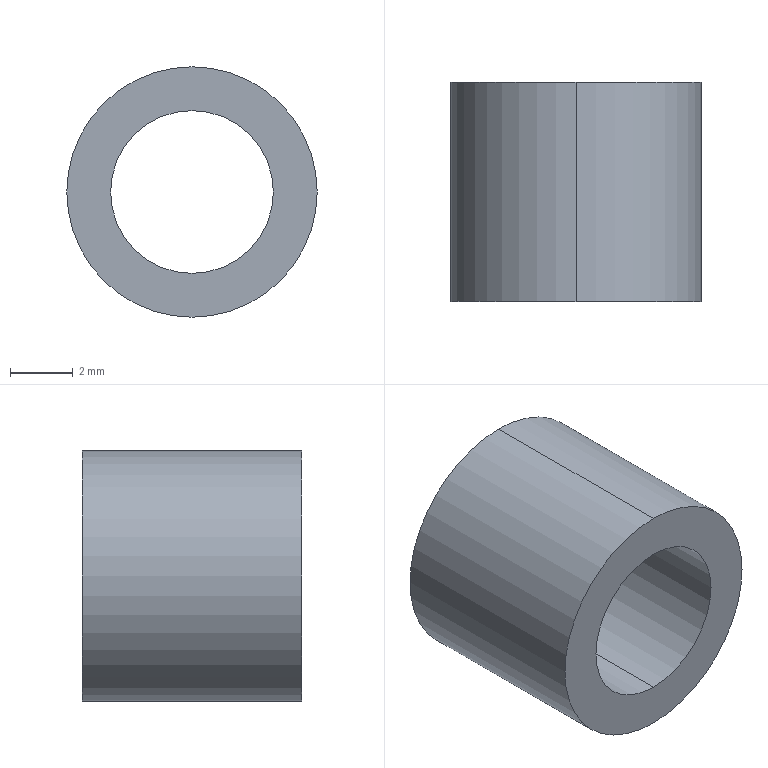Part | SolidWorks | features Extrusion 1 | 1 solid | 6 faces | box 8 x 7 x 8 mm | volume 203.198 mm3 | cylinder 4 | plane 2 | commonest cylinder face diameters 5.2 x2 8 x2
STEP:
#1=CARTESIAN_POINT('',(0.,7.,-2.6));
#2=VERTEX_POINT('',#1);
#3=CARTESIAN_POINT('',(0.,7.,2.6));
#4=VERTEX_POINT('',#3);
#5=CARTESIAN_POINT('',(0.,7.,0.));
#6=DIRECTION('',(0.,1.,0.));
#7=DIRECTION('',(0.,0.,1.));
#8=AXIS2_PLACEMENT_3D('',#5,#6,#7);
#9=CIRCLE('',#8,2.6);
#10=EDGE_CURVE('',#2,#4,#9,.T.);
#11=ORIENTED_EDGE('',*,*,#10,.T.);
#12=CARTESIAN_POINT('',(0.,0.,2.6));
#13=VERTEX_POINT('',#12);
#14=CARTESIAN_POINT('',(0.,7.,2.6));
#15=DIRECTION('',(0.,-1.,0.));
#16=VECTOR('',#15,1000.);
#17=LINE('',#14,#16);
#18=EDGE_CURVE('',#4,#13,#17,.T.);
#19=ORIENTED_EDGE('',*,*,#18,.T.);
#20=CARTESIAN_POINT('',(0.,0.,-2.6));
#21=VERTEX_POINT('',#20);
#22=CARTESIAN_POINT('',(0.,0.,0.));
#23=DIRECTION('',(0.,1.,0.));
#24=DIRECTION('',(0.,0.,1.));
#25=AXIS2_PLACEMENT_3D('',#22,#23,#24);
#26=CIRCLE('',#25,2.6);
#27=EDGE_CURVE('',#21,#13,#26,.T.);
#28=ORIENTED_EDGE('',*,*,#27,.F.);
#29=CARTESIAN_POINT('',(0.,7.,-2.6));
#30=DIRECTION('',(0.,-1.,0.));
#31=VECTOR('',#30,1000.);
#32=LINE('',#29,#31);
#33=EDGE_CURVE('',#2,#21,#32,.T.);
#34=ORIENTED_EDGE('',*,*,#33,.F.);
#35=EDGE_LOOP('',(#11,#19,#28,#34));
#36=FACE_OUTER_BOUND('',#35,.T.);
#37=CARTESIAN_POINT('',(0.,7.,0.));
#38=DIRECTION('',(0.,-1.,0.));
#39=DIRECTION('',(0.,0.,-1.));
#40=AXIS2_PLACEMENT_3D('',#37,#38,#39);
#41=CYLINDRICAL_SURFACE('',#40,2.6);
#42=ADVANCED_FACE('',(#36),#41,.F.);
#43=CARTESIAN_POINT('',(0.,7.,4.));
#44=VERTEX_POINT('',#43);
#45=CARTESIAN_POINT('',(0.,7.,-4.));
#46=VERTEX_POINT('',#45);
#47=CARTESIAN_POINT('',(0.,7.,0.));
#48=DIRECTION('',(0.,1.,0.));
#49=DIRECTION('',(0.,0.,1.));
#50=AXIS2_PLACEMENT_3D('',#47,#48,#49);
#51=CIRCLE('',#50,4.);
#52=EDGE_CURVE('',#44,#46,#51,.T.);
#53=ORIENTED_EDGE('',*,*,#52,.F.);
#54=CARTESIAN_POINT('',(0.,0.,4.));
#55=VERTEX_POINT('',#54);
#56=CARTESIAN_POINT('',(0.,7.,4.));
#57=DIRECTION('',(0.,-1.,0.));
#58=VECTOR('',#57,1000.);
#59=LINE('',#56,#58);
#60=EDGE_CURVE('',#44,#55,#59,.T.);
#61=ORIENTED_EDGE('',*,*,#60,.T.);
#62=CARTESIAN_POINT('',(0.,0.,-4.));
#63=VERTEX_POINT('',#62);
#64=CARTESIAN_POINT('',(0.,0.,0.));
#65=DIRECTION('',(0.,1.,0.));
#66=DIRECTION('',(0.,0.,1.));
#67=AXIS2_PLACEMENT_3D('',#64,#65,#66);
#68=CIRCLE('',#67,4.);
#69=EDGE_CURVE('',#55,#63,#68,.T.);
#70=ORIENTED_EDGE('',*,*,#69,.T.);
#71=CARTESIAN_POINT('',(0.,7.,-4.));
#72=DIRECTION('',(0.,-1.,0.));
#73=VECTOR('',#72,1000.);
#74=LINE('',#71,#73);
#75=EDGE_CURVE('',#46,#63,#74,.T.);
#76=ORIENTED_EDGE('',*,*,#75,.F.);
#77=EDGE_LOOP('',(#53,#61,#70,#76));
#78=FACE_OUTER_BOUND('',#77,.T.);
#79=CARTESIAN_POINT('',(0.,7.,0.));
#80=DIRECTION('',(0.,-1.,0.));
#81=DIRECTION('',(0.,0.,-1.));
#82=AXIS2_PLACEMENT_3D('',#79,#80,#81);
#83=CYLINDRICAL_SURFACE('',#82,4.);
#84=ADVANCED_FACE('',(#78),#83,.T.);
#85=CARTESIAN_POINT('',(0.,7.,0.));
#86=DIRECTION('',(0.,1.,0.));
#87=DIRECTION('',(0.,0.,1.));
#88=AXIS2_PLACEMENT_3D('',#85,#86,#87);
#89=CIRCLE('',#88,4.);
#90=EDGE_CURVE('',#46,#44,#89,.T.);
#91=ORIENTED_EDGE('',*,*,#90,.T.);
#92=ORIENTED_EDGE('',*,*,#52,.T.);
#93=EDGE_LOOP('',(#91,#92));
#94=FACE_OUTER_BOUND('',#93,.T.);
#95=ORIENTED_EDGE('',*,*,#10,.F.);
#96=CARTESIAN_POINT('',(0.,7.,0.));
#97=DIRECTION('',(0.,1.,0.));
#98=DIRECTION('',(0.,0.,1.));
#99=AXIS2_PLACEMENT_3D('',#96,#97,#98);
#100=CIRCLE('',#99,2.6);
#101=EDGE_CURVE('',#4,#2,#100,.T.);
#102=ORIENTED_EDGE('',*,*,#101,.F.);
#103=EDGE_LOOP('',(#95,#102));
#104=FACE_BOUND('',#103,.T.);
#105=CARTESIAN_POINT('',(0.,7.,0.));
#106=DIRECTION('',(0.,1.,0.));
#107=DIRECTION('',(0.,0.,1.));
#108=AXIS2_PLACEMENT_3D('',#105,#106,#107);
#109=PLANE('',#108);
#110=ADVANCED_FACE('',(#94,#104),#109,.T.);
#111=CARTESIAN_POINT('',(0.,0.,0.));
#112=DIRECTION('',(0.,1.,0.));
#113=DIRECTION('',(0.,0.,1.));
#114=AXIS2_PLACEMENT_3D('',#111,#112,#113);
#115=CIRCLE('',#114,4.);
#116=EDGE_CURVE('',#63,#55,#115,.T.);
#117=ORIENTED_EDGE('',*,*,#116,.F.);
#118=ORIENTED_EDGE('',*,*,#69,.F.);
#119=EDGE_LOOP('',(#117,#118));
#120=FACE_OUTER_BOUND('',#119,.T.);
#121=ORIENTED_EDGE('',*,*,#27,.T.);
#122=CARTESIAN_POINT('',(0.,0.,0.));
#123=DIRECTION('',(0.,1.,0.));
#124=DIRECTION('',(0.,0.,1.));
#125=AXIS2_PLACEMENT_3D('',#122,#123,#124);
#126=CIRCLE('',#125,2.6);
#127=EDGE_CURVE('',#13,#21,#126,.T.);
#128=ORIENTED_EDGE('',*,*,#127,.T.);
#129=EDGE_LOOP('',(#121,#128));
#130=FACE_BOUND('',#129,.T.);
#131=CARTESIAN_POINT('',(0.,0.,0.));
#132=DIRECTION('',(0.,1.,0.));
#133=DIRECTION('',(0.,0.,1.));
#134=AXIS2_PLACEMENT_3D('',#131,#132,#133);
#135=PLANE('',#134);
#136=ADVANCED_FACE('',(#120,#130),#135,.F.);
#137=ORIENTED_EDGE('',*,*,#60,.F.);
#138=ORIENTED_EDGE('',*,*,#90,.F.);
#139=ORIENTED_EDGE('',*,*,#75,.T.);
#140=ORIENTED_EDGE('',*,*,#116,.T.);
#141=EDGE_LOOP('',(#137,#138,#139,#140));
#142=FACE_OUTER_BOUND('',#141,.T.);
#143=CARTESIAN_POINT('',(0.,7.,0.));
#144=DIRECTION('',(0.,-1.,0.));
#145=DIRECTION('',(0.,0.,-1.));
#146=AXIS2_PLACEMENT_3D('',#143,#144,#145);
#147=CYLINDRICAL_SURFACE('',#146,4.);
#148=ADVANCED_FACE('',(#142),#147,.T.);
#149=ORIENTED_EDGE('',*,*,#18,.F.);
#150=ORIENTED_EDGE('',*,*,#101,.T.);
#151=ORIENTED_EDGE('',*,*,#33,.T.);
#152=ORIENTED_EDGE('',*,*,#127,.F.);
#153=EDGE_LOOP('',(#149,#150,#151,#152));
#154=FACE_OUTER_BOUND('',#153,.T.);
#155=CARTESIAN_POINT('',(0.,7.,0.));
#156=DIRECTION('',(0.,-1.,0.));
#157=DIRECTION('',(0.,0.,-1.));
#158=AXIS2_PLACEMENT_3D('',#155,#156,#157);
#159=CYLINDRICAL_SURFACE('',#158,2.6);
#160=ADVANCED_FACE('',(#154),#159,.F.);
#161=CLOSED_SHELL('',(#42,#84,#110,#136,#148,#160));
#162=MANIFOLD_SOLID_BREP('',#161);
#163=CARTESIAN_POINT('',(0.,0.,0.));
#164=DIRECTION('',(0.,0.,1.));
#165=DIRECTION('',(1.,0.,0.));
#166=AXIS2_PLACEMENT_3D('',#163,#164,#165);
#167=(LENGTH_UNIT()NAMED_UNIT(*)SI_UNIT(.MILLI.,.METRE.));
#168=UNCERTAINTY_MEASURE_WITH_UNIT(LENGTH_MEASURE(0.00001),#167,'','');
#169=(NAMED_UNIT(*)PLANE_ANGLE_UNIT()SI_UNIT($,.RADIAN.));
#170=(NAMED_UNIT(*)SI_UNIT($,.STERADIAN.)SOLID_ANGLE_UNIT());
#171=(GEOMETRIC_REPRESENTATION_CONTEXT(3)GLOBAL_UNCERTAINTY_ASSIGNED_CONTEXT((#168))GLOBAL_UNIT_ASSIGNED_CONTEXT((#167,#169,#170))REPRESENTATION_CONTEXT('',''));
#172=ADVANCED_BREP_SHAPE_REPRESENTATION('',(#162,#166),#171);